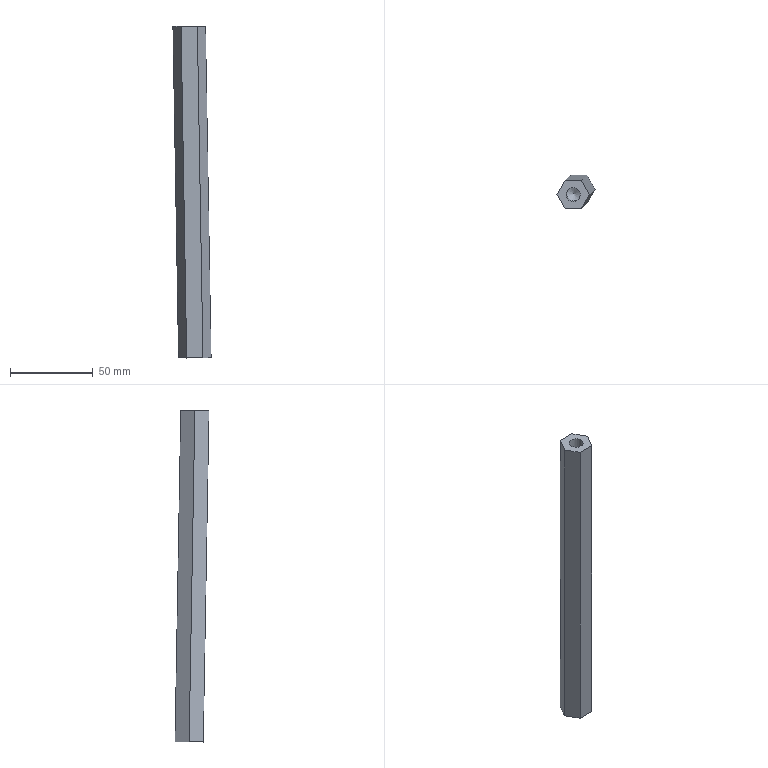Part | NX | features B0 2 | 1 solid | 12 faces | box 23.011 x 20.454 x 200.401 mm | volume 47179 mm3 | plane 8 | cone 2 | cylinder 2 | commonest cylinder face diameters 8.5 x2
STEP:
#1=CARTESIAN_POINT('',(3.484,50.556,-587.886));
#2=VERTEX_POINT('',#1);
#3=VERTEX_LOOP('',#2);
#4=FACE_BOUND('',#3,.T.);
#5=CARTESIAN_POINT('',(5.652,46.92,-590.467));
#6=VERTEX_POINT('',#5);
#7=CARTESIAN_POINT('',(3.527,50.6,-590.439));
#8=DIRECTION('',(0.01692,0.01727,-0.9997));
#9=DIRECTION('',(0.4999,-0.866,-0.006499));
#10=AXIS2_PLACEMENT_3D('',#7,#8,#9);
#11=CIRCLE('',#10,4.25);
#12=EDGE_CURVE('',#6,#6,#11,.T.);
#13=ORIENTED_EDGE('',*,*,#12,.T.);
#14=EDGE_LOOP('',(#13));
#15=FACE_BOUND('',#14,.T.);
#16=CARTESIAN_POINT('',(3.484,50.556,-587.886));
#17=DIRECTION('',(0.01692,0.01727,-0.9997));
#18=DIRECTION('',(0.4999,-0.866,-0.006499));
#19=AXIS2_PLACEMENT_3D('',#16,#17,#18);
#20=CONICAL_SURFACE('',#19,0.,1.03);
#21=ADVANCED_FACE('',(#4,#15),#20,.F.);
#22=ORIENTED_EDGE('',*,*,#12,.F.);
#23=EDGE_LOOP('',(#22));
#24=FACE_BOUND('',#23,.T.);
#25=CARTESIAN_POINT('',(1.817,54.704,-614.904));
#26=VERTEX_POINT('',#25);
#27=CARTESIAN_POINT('',(3.942,51.023,-614.932));
#28=DIRECTION('',(-0.01692,-0.01727,0.9997));
#29=DIRECTION('',(-0.4999,0.866,0.006499));
#30=AXIS2_PLACEMENT_3D('',#27,#28,#29);
#31=CIRCLE('',#30,4.25);
#32=EDGE_CURVE('',#26,#26,#31,.T.);
#33=ORIENTED_EDGE('',*,*,#32,.F.);
#34=EDGE_LOOP('',(#33));
#35=FACE_BOUND('',#34,.T.);
#36=CARTESIAN_POINT('',(3.942,51.023,-614.932));
#37=DIRECTION('',(0.01692,0.01727,-0.9997));
#38=DIRECTION('',(0.4999,-0.866,-0.006499));
#39=AXIS2_PLACEMENT_3D('',#36,#37,#38);
#40=CYLINDRICAL_SURFACE('',#39,4.25);
#41=ADVANCED_FACE('',(#24,#35),#40,.F.);
#42=CARTESIAN_POINT('',(8.849,59.521,-614.702));
#43=VERTEX_POINT('',#42);
#44=CARTESIAN_POINT('',(5.465,56.067,-414.761));
#45=VERTEX_POINT('',#44);
#46=CARTESIAN_POINT('',(8.849,59.521,-614.702));
#47=DIRECTION('',(-0.01692,-0.01727,0.9997));
#48=VECTOR('',#47,1000.);
#49=LINE('',#46,#48);
#50=EDGE_CURVE('',#43,#45,#49,.T.);
#51=ORIENTED_EDGE('',*,*,#50,.T.);
#52=CARTESIAN_POINT('',(10.372,47.567,-414.824));
#53=VERTEX_POINT('',#52);
#54=CARTESIAN_POINT('',(5.465,56.067,-414.761));
#55=DIRECTION('',(0.4999,-0.866,-0.006499));
#56=VECTOR('',#55,1000.);
#57=LINE('',#54,#56);
#58=EDGE_CURVE('',#45,#53,#57,.T.);
#59=ORIENTED_EDGE('',*,*,#58,.T.);
#60=CARTESIAN_POINT('',(13.755,51.021,-614.766));
#61=VERTEX_POINT('',#60);
#62=CARTESIAN_POINT('',(13.755,51.021,-614.766));
#63=DIRECTION('',(-0.01692,-0.01727,0.9997));
#64=VECTOR('',#63,1000.);
#65=LINE('',#62,#64);
#66=EDGE_CURVE('',#61,#53,#65,.T.);
#67=ORIENTED_EDGE('',*,*,#66,.F.);
#68=CARTESIAN_POINT('',(8.849,59.521,-614.702));
#69=DIRECTION('',(0.4999,-0.866,-0.006499));
#70=VECTOR('',#69,1000.);
#71=LINE('',#68,#70);
#72=EDGE_CURVE('',#43,#61,#71,.T.);
#73=ORIENTED_EDGE('',*,*,#72,.F.);
#74=EDGE_LOOP('',(#51,#59,#67,#73));
#75=FACE_BOUND('',#74,.T.);
#76=CARTESIAN_POINT('',(10.372,47.567,-414.824));
#77=DIRECTION('',(-0.8659,-0.4997,-0.02328));
#78=DIRECTION('',(-0.01692,-0.01727,0.9997));
#79=AXIS2_PLACEMENT_3D('',#76,#77,#78);
#80=PLANE('',#79);
#81=ADVANCED_FACE('',(#75),#80,.F.);
#82=ORIENTED_EDGE('',*,*,#66,.T.);
#83=CARTESIAN_POINT('',(5.465,39.07,-415.054));
#84=VERTEX_POINT('',#83);
#85=CARTESIAN_POINT('',(5.465,39.07,-415.054));
#86=DIRECTION('',(0.4999,0.8658,0.02341));
#87=VECTOR('',#86,1000.);
#88=LINE('',#85,#87);
#89=EDGE_CURVE('',#84,#53,#88,.T.);
#90=ORIENTED_EDGE('',*,*,#89,.F.);
#91=CARTESIAN_POINT('',(8.849,42.523,-614.996));
#92=VERTEX_POINT('',#91);
#93=CARTESIAN_POINT('',(8.849,42.523,-614.996));
#94=DIRECTION('',(-0.01692,-0.01727,0.9997));
#95=VECTOR('',#94,1000.);
#96=LINE('',#93,#95);
#97=EDGE_CURVE('',#92,#84,#96,.T.);
#98=ORIENTED_EDGE('',*,*,#97,.F.);
#99=CARTESIAN_POINT('',(13.755,51.021,-614.766));
#100=DIRECTION('',(-0.4999,-0.8658,-0.02341));
#101=VECTOR('',#100,1000.);
#102=LINE('',#99,#101);
#103=EDGE_CURVE('',#61,#92,#102,.T.);
#104=ORIENTED_EDGE('',*,*,#103,.F.);
#105=EDGE_LOOP('',(#82,#90,#98,#104));
#106=FACE_BOUND('',#105,.T.);
#107=CARTESIAN_POINT('',(5.465,39.07,-415.054));
#108=DIRECTION('',(-0.8659,0.5002,-0.006013));
#109=DIRECTION('',(-0.4999,-0.8658,-0.02341));
#110=AXIS2_PLACEMENT_3D('',#107,#108,#109);
#111=PLANE('',#110);
#112=ADVANCED_FACE('',(#106),#111,.F.);
#113=ORIENTED_EDGE('',*,*,#97,.T.);
#114=CARTESIAN_POINT('',(-4.349,39.073,-415.22));
#115=VERTEX_POINT('',#114);
#116=CARTESIAN_POINT('',(-4.349,39.073,-415.22));
#117=DIRECTION('',(0.9999,-0.0002922,0.01691));
#118=VECTOR('',#117,1000.);
#119=LINE('',#116,#118);
#120=EDGE_CURVE('',#115,#84,#119,.T.);
#121=ORIENTED_EDGE('',*,*,#120,.F.);
#122=CARTESIAN_POINT('',(-0.965,42.526,-615.162));
#123=VERTEX_POINT('',#122);
#124=CARTESIAN_POINT('',(-0.965,42.526,-615.162));
#125=DIRECTION('',(-0.01692,-0.01727,0.9997));
#126=VECTOR('',#125,1000.);
#127=LINE('',#124,#126);
#128=EDGE_CURVE('',#123,#115,#127,.T.);
#129=ORIENTED_EDGE('',*,*,#128,.F.);
#130=CARTESIAN_POINT('',(8.849,42.523,-614.996));
#131=DIRECTION('',(-0.9999,0.0002922,-0.01691));
#132=VECTOR('',#131,1000.);
#133=LINE('',#130,#132);
#134=EDGE_CURVE('',#92,#123,#133,.T.);
#135=ORIENTED_EDGE('',*,*,#134,.F.);
#136=EDGE_LOOP('',(#113,#121,#129,#135));
#137=FACE_BOUND('',#136,.T.);
#138=CARTESIAN_POINT('',(-4.349,39.073,-415.22));
#139=DIRECTION('',(0.,0.9999,0.01727));
#140=DIRECTION('',(-0.9999,0.0002922,-0.01691));
#141=AXIS2_PLACEMENT_3D('',#138,#139,#140);
#142=PLANE('',#141);
#143=ADVANCED_FACE('',(#137),#142,.F.);
#144=ORIENTED_EDGE('',*,*,#128,.T.);
#145=CARTESIAN_POINT('',(-9.255,47.573,-415.156));
#146=VERTEX_POINT('',#145);
#147=CARTESIAN_POINT('',(-4.349,39.073,-415.22));
#148=DIRECTION('',(-0.4999,0.866,0.006499));
#149=VECTOR('',#148,1000.);
#150=LINE('',#147,#149);
#151=EDGE_CURVE('',#115,#146,#150,.T.);
#152=ORIENTED_EDGE('',*,*,#151,.T.);
#153=CARTESIAN_POINT('',(-5.872,51.026,-615.098));
#154=VERTEX_POINT('',#153);
#155=CARTESIAN_POINT('',(-5.872,51.026,-615.098));
#156=DIRECTION('',(-0.01692,-0.01727,0.9997));
#157=VECTOR('',#156,1000.);
#158=LINE('',#155,#157);
#159=EDGE_CURVE('',#154,#146,#158,.T.);
#160=ORIENTED_EDGE('',*,*,#159,.F.);
#161=CARTESIAN_POINT('',(-0.965,42.526,-615.162));
#162=DIRECTION('',(-0.4999,0.866,0.006499));
#163=VECTOR('',#162,1000.);
#164=LINE('',#161,#163);
#165=EDGE_CURVE('',#123,#154,#164,.T.);
#166=ORIENTED_EDGE('',*,*,#165,.F.);
#167=EDGE_LOOP('',(#144,#152,#160,#166));
#168=FACE_BOUND('',#167,.T.);
#169=CARTESIAN_POINT('',(-9.255,47.573,-415.156));
#170=DIRECTION('',(0.8659,0.4997,0.02328));
#171=DIRECTION('',(-0.4999,0.866,0.006499));
#172=AXIS2_PLACEMENT_3D('',#169,#170,#171);
#173=PLANE('',#172);
#174=ADVANCED_FACE('',(#168),#173,.F.);
#175=ORIENTED_EDGE('',*,*,#159,.T.);
#176=CARTESIAN_POINT('',(-4.349,56.07,-414.927));
#177=VERTEX_POINT('',#176);
#178=CARTESIAN_POINT('',(-4.349,56.07,-414.927));
#179=DIRECTION('',(-0.4999,-0.8658,-0.02341));
#180=VECTOR('',#179,1000.);
#181=LINE('',#178,#180);
#182=EDGE_CURVE('',#177,#146,#181,.T.);
#183=ORIENTED_EDGE('',*,*,#182,.F.);
#184=CARTESIAN_POINT('',(-0.965,59.524,-614.868));
#185=VERTEX_POINT('',#184);
#186=CARTESIAN_POINT('',(-0.965,59.524,-614.868));
#187=DIRECTION('',(-0.01692,-0.01727,0.9997));
#188=VECTOR('',#187,1000.);
#189=LINE('',#186,#188);
#190=EDGE_CURVE('',#185,#177,#189,.T.);
#191=ORIENTED_EDGE('',*,*,#190,.F.);
#192=CARTESIAN_POINT('',(-5.872,51.026,-615.098));
#193=DIRECTION('',(0.4999,0.8658,0.02341));
#194=VECTOR('',#193,1000.);
#195=LINE('',#192,#194);
#196=EDGE_CURVE('',#154,#185,#195,.T.);
#197=ORIENTED_EDGE('',*,*,#196,.F.);
#198=EDGE_LOOP('',(#175,#183,#191,#197));
#199=FACE_BOUND('',#198,.T.);
#200=CARTESIAN_POINT('',(-4.349,56.07,-414.927));
#201=DIRECTION('',(0.8659,-0.5002,0.006013));
#202=DIRECTION('',(0.4999,0.8658,0.02341));
#203=AXIS2_PLACEMENT_3D('',#200,#201,#202);
#204=PLANE('',#203);
#205=ADVANCED_FACE('',(#199),#204,.F.);
#206=ORIENTED_EDGE('',*,*,#32,.T.);
#207=EDGE_LOOP('',(#206));
#208=FACE_BOUND('',#207,.T.);
#209=ORIENTED_EDGE('',*,*,#72,.T.);
#210=ORIENTED_EDGE('',*,*,#103,.T.);
#211=ORIENTED_EDGE('',*,*,#134,.T.);
#212=ORIENTED_EDGE('',*,*,#165,.T.);
#213=ORIENTED_EDGE('',*,*,#196,.T.);
#214=CARTESIAN_POINT('',(-0.965,59.524,-614.868));
#215=DIRECTION('',(0.9999,-0.0002922,0.01691));
#216=VECTOR('',#215,1000.);
#217=LINE('',#214,#216);
#218=EDGE_CURVE('',#185,#43,#217,.T.);
#219=ORIENTED_EDGE('',*,*,#218,.T.);
#220=EDGE_LOOP('',(#209,#210,#211,#212,#213,#219));
#221=FACE_BOUND('',#220,.T.);
#222=CARTESIAN_POINT('',(3.942,51.023,-614.932));
#223=DIRECTION('',(-0.01692,-0.01727,0.9997));
#224=DIRECTION('',(-0.4999,0.866,0.006499));
#225=AXIS2_PLACEMENT_3D('',#222,#223,#224);
#226=PLANE('',#225);
#227=ADVANCED_FACE('',(#208,#221),#226,.F.);
#228=ORIENTED_EDGE('',*,*,#190,.T.);
#229=CARTESIAN_POINT('',(5.465,56.067,-414.761));
#230=DIRECTION('',(-0.9999,0.0002922,-0.01691));
#231=VECTOR('',#230,1000.);
#232=LINE('',#229,#231);
#233=EDGE_CURVE('',#45,#177,#232,.T.);
#234=ORIENTED_EDGE('',*,*,#233,.F.);
#235=ORIENTED_EDGE('',*,*,#50,.F.);
#236=ORIENTED_EDGE('',*,*,#218,.F.);
#237=EDGE_LOOP('',(#228,#234,#235,#236));
#238=FACE_BOUND('',#237,.T.);
#239=CARTESIAN_POINT('',(5.465,56.067,-414.761));
#240=DIRECTION('',(0.,-0.9999,-0.01727));
#241=DIRECTION('',(0.9999,-0.0002922,0.01691));
#242=AXIS2_PLACEMENT_3D('',#239,#240,#241);
#243=PLANE('',#242);
#244=ADVANCED_FACE('',(#238),#243,.F.);
#245=CARTESIAN_POINT('',(-1.566,51.251,-414.963));
#246=VERTEX_POINT('',#245);
#247=CARTESIAN_POINT('',(0.5583,47.57,-414.99));
#248=DIRECTION('',(0.01692,0.01727,-0.9997));
#249=DIRECTION('',(-0.4999,0.866,0.006499));
#250=AXIS2_PLACEMENT_3D('',#247,#248,#249);
#251=CIRCLE('',#250,4.25);
#252=EDGE_CURVE('',#246,#246,#251,.T.);
#253=ORIENTED_EDGE('',*,*,#252,.T.);
#254=EDGE_LOOP('',(#253));
#255=FACE_BOUND('',#254,.T.);
#256=ORIENTED_EDGE('',*,*,#182,.T.);
#257=ORIENTED_EDGE('',*,*,#151,.F.);
#258=ORIENTED_EDGE('',*,*,#120,.T.);
#259=ORIENTED_EDGE('',*,*,#89,.T.);
#260=ORIENTED_EDGE('',*,*,#58,.F.);
#261=ORIENTED_EDGE('',*,*,#233,.T.);
#262=EDGE_LOOP('',(#256,#257,#258,#259,#260,#261));
#263=FACE_BOUND('',#262,.T.);
#264=CARTESIAN_POINT('',(0.5583,47.57,-414.99));
#265=DIRECTION('',(-0.01692,-0.01727,0.9997));
#266=DIRECTION('',(-0.4999,0.866,0.006499));
#267=AXIS2_PLACEMENT_3D('',#264,#265,#266);
#268=PLANE('',#267);
#269=ADVANCED_FACE('',(#255,#263),#268,.T.);
#270=CARTESIAN_POINT('',(-1.152,51.674,-439.456));
#271=VERTEX_POINT('',#270);
#272=CARTESIAN_POINT('',(0.9727,47.993,-439.483));
#273=DIRECTION('',(-0.01692,-0.01727,0.9997));
#274=DIRECTION('',(-0.4999,0.866,0.006499));
#275=AXIS2_PLACEMENT_3D('',#272,#273,#274);
#276=CIRCLE('',#275,4.25);
#277=EDGE_CURVE('',#271,#271,#276,.T.);
#278=ORIENTED_EDGE('',*,*,#277,.F.);
#279=EDGE_LOOP('',(#278));
#280=FACE_BOUND('',#279,.T.);
#281=ORIENTED_EDGE('',*,*,#252,.F.);
#282=EDGE_LOOP('',(#281));
#283=FACE_BOUND('',#282,.T.);
#284=CARTESIAN_POINT('',(0.5583,47.57,-414.99));
#285=DIRECTION('',(-0.01692,-0.01727,0.9997));
#286=DIRECTION('',(-0.4999,0.866,0.006499));
#287=AXIS2_PLACEMENT_3D('',#284,#285,#286);
#288=CYLINDRICAL_SURFACE('',#287,4.25);
#289=ADVANCED_FACE('',(#280,#283),#288,.F.);
#290=CARTESIAN_POINT('',(1.016,48.037,-442.036));
#291=VERTEX_POINT('',#290);
#292=VERTEX_LOOP('',#291);
#293=FACE_BOUND('',#292,.T.);
#294=ORIENTED_EDGE('',*,*,#277,.T.);
#295=EDGE_LOOP('',(#294));
#296=FACE_BOUND('',#295,.T.);
#297=CARTESIAN_POINT('',(1.016,48.037,-442.036));
#298=DIRECTION('',(-0.01692,-0.01727,0.9997));
#299=DIRECTION('',(-0.4999,0.866,0.006499));
#300=AXIS2_PLACEMENT_3D('',#297,#298,#299);
#301=CONICAL_SURFACE('',#300,0.,1.03);
#302=ADVANCED_FACE('',(#293,#296),#301,.F.);
#303=CLOSED_SHELL('',(#21,#41,#81,#112,#143,#174,#205,#227,#244,#269,#289,#302));
#304=MANIFOLD_SOLID_BREP('',#303);
#305=(LENGTH_UNIT()NAMED_UNIT(*)SI_UNIT(.MILLI.,.METRE.));
#306=UNCERTAINTY_MEASURE_WITH_UNIT(LENGTH_MEASURE(0.00001),#305,'','');
#307=(NAMED_UNIT(*)PLANE_ANGLE_UNIT()SI_UNIT($,.RADIAN.));
#308=(NAMED_UNIT(*)SI_UNIT($,.STERADIAN.)SOLID_ANGLE_UNIT());
#309=(GEOMETRIC_REPRESENTATION_CONTEXT(3)GLOBAL_UNCERTAINTY_ASSIGNED_CONTEXT((#306))GLOBAL_UNIT_ASSIGNED_CONTEXT((#305,#307,#308))REPRESENTATION_CONTEXT('',''));
#310=ADVANCED_BREP_SHAPE_REPRESENTATION('',(#304),#309);